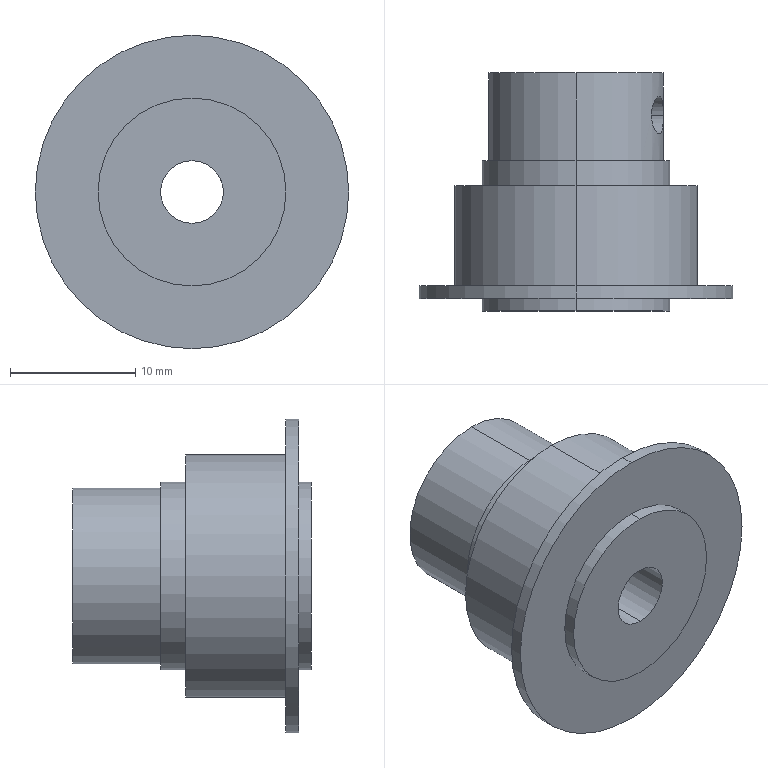Part | SolidWorks | features 3DProfileFeature 1, BaseBody 1, HoleWzd 1 | 1 solid | 20 faces | box 25 x 19 x 25 mm | volume 4058 mm3 | cylinder 14 | plane 6 | commonest cylinder face diameters 15 x4 3 x2 5 x2 14 x2 19.4 x2 25 x2
STEP:
#1=CARTESIAN_POINT('',(1.426,14.633,2.053));
#2=VERTEX_POINT('',#1);
#3=CARTESIAN_POINT('',(2.37,14.633,-0.7943));
#4=VERTEX_POINT('',#3);
#5=CARTESIAN_POINT('',(1.426,14.633,2.053));
#6=CARTESIAN_POINT('',(1.426,14.531,2.053));
#7=CARTESIAN_POINT('',(1.437,14.431,2.046));
#8=CARTESIAN_POINT('',(1.477,14.236,2.017));
#9=CARTESIAN_POINT('',(1.506,14.14,1.996));
#10=CARTESIAN_POINT('',(1.614,13.87,1.912));
#11=CARTESIAN_POINT('',(1.711,13.709,1.829));
#12=CARTESIAN_POINT('',(1.865,13.506,1.666));
#13=CARTESIAN_POINT('',(1.919,13.444,1.605));
#14=CARTESIAN_POINT('',(2.023,13.336,1.471));
#15=CARTESIAN_POINT('',(2.074,13.29,1.399));
#16=CARTESIAN_POINT('',(2.173,13.213,1.24));
#17=CARTESIAN_POINT('',(2.22,13.183,1.155));
#18=CARTESIAN_POINT('',(2.303,13.143,0.9773));
#19=CARTESIAN_POINT('',(2.341,13.133,0.8843));
#20=CARTESIAN_POINT('',(2.405,13.133,0.6911));
#21=CARTESIAN_POINT('',(2.43,13.143,0.5944));
#22=CARTESIAN_POINT('',(2.47,13.183,0.401));
#23=CARTESIAN_POINT('',(2.483,13.213,0.3036));
#24=CARTESIAN_POINT('',(2.507,13.328,0.0251));
#25=CARTESIAN_POINT('',(2.5,13.439,-0.1488));
#26=CARTESIAN_POINT('',(2.473,13.642,-0.3709));
#27=CARTESIAN_POINT('',(2.462,13.717,-0.4397));
#28=CARTESIAN_POINT('',(2.437,13.876,-0.5603));
#29=CARTESIAN_POINT('',(2.424,13.961,-0.6128));
#30=CARTESIAN_POINT('',(2.4,14.141,-0.7006));
#31=CARTESIAN_POINT('',(2.389,14.237,-0.7355));
#32=CARTESIAN_POINT('',(2.375,14.431,-0.782));
#33=CARTESIAN_POINT('',(2.37,14.531,-0.7943));
#34=CARTESIAN_POINT('',(2.37,14.633,-0.7943));
#35=B_SPLINE_CURVE_WITH_KNOTS('',3,(#5,#6,#7,#8,#9,#10,#11,#12,#13,#14,#15,#16,#17,#18,#19,#20,#21,#22,#23,#24,#25,#26,#27,#28,#29,#30,#31,#32,#33,#34),.UNSPECIFIED.,.F.,.F.,(4,2,2,2,2,2,2,2,2,2,2,2,2,2,4),(0.00481,0.00511,0.005411,0.006011,0.006311,0.006611,0.006911,0.007211,0.007511,0.007811,0.008412,0.008712,0.009012,0.009312,0.009612),.UNSPECIFIED.);
#36=EDGE_CURVE('',#2,#4,#35,.T.);
#37=ORIENTED_EDGE('',*,*,#36,.F.);
#38=CARTESIAN_POINT('',(6.018,14.633,3.576));
#39=VERTEX_POINT('',#38);
#40=CARTESIAN_POINT('',(6.172,14.633,3.627));
#41=DIRECTION('',(0.9492,0.,0.3147));
#42=VECTOR('',#41,1000.);
#43=LINE('',#40,#42);
#44=EDGE_CURVE('',#2,#39,#43,.T.);
#45=ORIENTED_EDGE('',*,*,#44,.T.);
#46=CARTESIAN_POINT('',(6.962,14.633,0.7282));
#47=VERTEX_POINT('',#46);
#48=CARTESIAN_POINT('',(6.962,14.633,0.7282));
#49=CARTESIAN_POINT('',(6.962,14.533,0.7282));
#50=CARTESIAN_POINT('',(6.961,14.436,0.7382));
#51=CARTESIAN_POINT('',(6.957,14.244,0.7771));
#52=CARTESIAN_POINT('',(6.953,14.148,0.8065));
#53=CARTESIAN_POINT('',(6.944,13.967,0.8829));
#54=CARTESIAN_POINT('',(6.938,13.881,0.9295));
#55=CARTESIAN_POINT('',(6.923,13.718,1.039));
#56=CARTESIAN_POINT('',(6.913,13.641,1.102));
#57=CARTESIAN_POINT('',(6.878,13.434,1.309));
#58=CARTESIAN_POINT('',(6.845,13.322,1.474));
#59=CARTESIAN_POINT('',(6.76,13.173,1.826));
#60=CARTESIAN_POINT('',(6.706,13.133,2.016));
#61=CARTESIAN_POINT('',(6.614,13.133,2.296));
#62=CARTESIAN_POINT('',(6.58,13.143,2.39));
#63=CARTESIAN_POINT('',(6.512,13.181,2.57));
#64=CARTESIAN_POINT('',(6.477,13.209,2.657));
#65=CARTESIAN_POINT('',(6.37,13.323,2.909));
#66=CARTESIAN_POINT('',(6.298,13.433,3.059));
#67=CARTESIAN_POINT('',(6.202,13.642,3.247));
#68=CARTESIAN_POINT('',(6.172,13.717,3.303));
#69=CARTESIAN_POINT('',(6.119,13.88,3.4));
#70=CARTESIAN_POINT('',(6.096,13.967,3.441));
#71=CARTESIAN_POINT('',(6.058,14.149,3.508));
#72=CARTESIAN_POINT('',(6.043,14.242,3.533));
#73=CARTESIAN_POINT('',(6.023,14.435,3.567));
#74=CARTESIAN_POINT('',(6.018,14.535,3.576));
#75=CARTESIAN_POINT('',(6.018,14.633,3.576));
#76=B_SPLINE_CURVE_WITH_KNOTS('',3,(#48,#49,#50,#51,#52,#53,#54,#55,#56,#57,#58,#59,#60,#61,#62,#63,#64,#65,#66,#67,#68,#69,#70,#71,#72,#73,#74,#75),.UNSPECIFIED.,.F.,.F.,(4,2,2,2,2,2,2,2,2,2,2,2,2,4),(0.,0.000294,0.0005879,0.0008819,0.001176,0.001764,0.002352,0.002646,0.00294,0.003527,0.003821,0.004115,0.004409,0.004703),.UNSPECIFIED.);
#77=EDGE_CURVE('',#47,#39,#76,.T.);
#78=ORIENTED_EDGE('',*,*,#77,.F.);
#79=CARTESIAN_POINT('',(7.116,14.633,0.7794));
#80=DIRECTION('',(0.9492,0.,0.3147));
#81=VECTOR('',#80,1000.);
#82=LINE('',#79,#81);
#83=EDGE_CURVE('',#4,#47,#82,.T.);
#84=ORIENTED_EDGE('',*,*,#83,.F.);
#85=EDGE_LOOP('',(#37,#45,#78,#84));
#86=FACE_OUTER_BOUND('',#85,.T.);
#87=CARTESIAN_POINT('',(6.644,14.633,2.203));
#88=DIRECTION('',(0.9492,0.,0.3147));
#89=DIRECTION('',(0.3147,0.,-0.9492));
#90=AXIS2_PLACEMENT_3D('',#87,#88,#89);
#91=CYLINDRICAL_SURFACE('',#90,1.5);
#92=ADVANCED_FACE('',(#86),#91,.F.);
#93=CARTESIAN_POINT('',(0.,-1.,-2.5));
#94=VERTEX_POINT('',#93);
#95=CARTESIAN_POINT('',(0.,-1.,2.5));
#96=VERTEX_POINT('',#95);
#97=CARTESIAN_POINT('',(0.,-1.,0.));
#98=DIRECTION('',(0.,1.,0.));
#99=DIRECTION('',(0.,0.,1.));
#100=AXIS2_PLACEMENT_3D('',#97,#98,#99);
#101=CIRCLE('',#100,2.5);
#102=EDGE_CURVE('',#94,#96,#101,.T.);
#103=ORIENTED_EDGE('',*,*,#102,.F.);
#104=CARTESIAN_POINT('',(0.,18.,-2.5));
#105=VERTEX_POINT('',#104);
#106=CARTESIAN_POINT('',(0.,-1.,-2.5));
#107=DIRECTION('',(0.,1.,0.));
#108=VECTOR('',#107,1000.);
#109=LINE('',#106,#108);
#110=EDGE_CURVE('',#94,#105,#109,.T.);
#111=ORIENTED_EDGE('',*,*,#110,.T.);
#112=CARTESIAN_POINT('',(0.,18.,2.5));
#113=VERTEX_POINT('',#112);
#114=CARTESIAN_POINT('',(0.,18.,0.));
#115=DIRECTION('',(0.,1.,0.));
#116=DIRECTION('',(0.,0.,1.));
#117=AXIS2_PLACEMENT_3D('',#114,#115,#116);
#118=CIRCLE('',#117,2.5);
#119=EDGE_CURVE('',#105,#113,#118,.T.);
#120=ORIENTED_EDGE('',*,*,#119,.T.);
#121=CARTESIAN_POINT('',(0.,-1.,2.5));
#122=DIRECTION('',(0.,1.,0.));
#123=VECTOR('',#122,1000.);
#124=LINE('',#121,#123);
#125=EDGE_CURVE('',#96,#113,#124,.T.);
#126=ORIENTED_EDGE('',*,*,#125,.F.);
#127=EDGE_LOOP('',(#103,#111,#120,#126));
#128=FACE_OUTER_BOUND('',#127,.T.);
#129=CARTESIAN_POINT('',(0.,-1.,0.));
#130=DIRECTION('',(0.,1.,0.));
#131=DIRECTION('',(0.,0.,1.));
#132=AXIS2_PLACEMENT_3D('',#129,#130,#131);
#133=CYLINDRICAL_SURFACE('',#132,2.5);
#134=ADVANCED_FACE('',(#128),#133,.F.);
#135=ORIENTED_EDGE('',*,*,#77,.T.);
#136=CARTESIAN_POINT('',(6.018,14.633,3.576));
#137=CARTESIAN_POINT('',(6.018,14.829,3.576));
#138=CARTESIAN_POINT('',(6.039,15.027,3.541));
#139=CARTESIAN_POINT('',(6.115,15.388,3.408));
#140=CARTESIAN_POINT('',(6.17,15.555,3.309));
#141=CARTESIAN_POINT('',(6.265,15.762,3.123));
#142=CARTESIAN_POINT('',(6.3,15.825,3.053));
#143=CARTESIAN_POINT('',(6.369,15.934,2.905));
#144=CARTESIAN_POINT('',(6.405,15.98,2.826));
#145=CARTESIAN_POINT('',(6.512,16.094,2.574));
#146=CARTESIAN_POINT('',(6.582,16.133,2.392));
#147=CARTESIAN_POINT('',(6.675,16.133,2.11));
#148=CARTESIAN_POINT('',(6.704,16.123,2.017));
#149=CARTESIAN_POINT('',(6.757,16.085,1.831));
#150=CARTESIAN_POINT('',(6.781,16.056,1.739));
#151=CARTESIAN_POINT('',(6.846,15.943,1.474));
#152=CARTESIAN_POINT('',(6.878,15.832,1.309));
#153=CARTESIAN_POINT('',(6.925,15.556,1.034));
#154=CARTESIAN_POINT('',(6.94,15.39,0.9212));
#155=CARTESIAN_POINT('',(6.958,15.029,0.7691));
#156=CARTESIAN_POINT('',(6.962,14.832,0.7282));
#157=CARTESIAN_POINT('',(6.962,14.633,0.7282));
#158=B_SPLINE_CURVE_WITH_KNOTS('',3,(#136,#137,#138,#139,#140,#141,#142,#143,#144,#145,#146,#147,#148,#149,#150,#151,#152,#153,#154,#155,#156,#157),.UNSPECIFIED.,.F.,.F.,(4,2,2,2,2,2,2,2,2,2,4),(0.004703,0.005291,0.005879,0.006173,0.006467,0.007054,0.007348,0.007642,0.00823,0.008818,0.009405),.UNSPECIFIED.);
#159=EDGE_CURVE('',#39,#47,#158,.T.);
#160=ORIENTED_EDGE('',*,*,#159,.T.);
#161=EDGE_LOOP('',(#135,#160));
#162=FACE_BOUND('',#161,.T.);
#163=CARTESIAN_POINT('',(0.,18.,7.));
#164=VERTEX_POINT('',#163);
#165=CARTESIAN_POINT('',(0.,18.,-7.));
#166=VERTEX_POINT('',#165);
#167=CARTESIAN_POINT('',(0.,18.,0.));
#168=DIRECTION('',(0.,1.,0.));
#169=DIRECTION('',(0.,0.,1.));
#170=AXIS2_PLACEMENT_3D('',#167,#168,#169);
#171=CIRCLE('',#170,7.);
#172=EDGE_CURVE('',#164,#166,#171,.T.);
#173=ORIENTED_EDGE('',*,*,#172,.F.);
#174=CARTESIAN_POINT('',(0.,11.,7.));
#175=VERTEX_POINT('',#174);
#176=CARTESIAN_POINT('',(0.,18.,7.));
#177=DIRECTION('',(0.,-1.,0.));
#178=VECTOR('',#177,1000.);
#179=LINE('',#176,#178);
#180=EDGE_CURVE('',#164,#175,#179,.T.);
#181=ORIENTED_EDGE('',*,*,#180,.T.);
#182=CARTESIAN_POINT('',(0.,11.,-7.));
#183=VERTEX_POINT('',#182);
#184=CARTESIAN_POINT('',(0.,11.,0.));
#185=DIRECTION('',(0.,1.,0.));
#186=DIRECTION('',(0.,0.,1.));
#187=AXIS2_PLACEMENT_3D('',#184,#185,#186);
#188=CIRCLE('',#187,7.);
#189=EDGE_CURVE('',#175,#183,#188,.T.);
#190=ORIENTED_EDGE('',*,*,#189,.T.);
#191=CARTESIAN_POINT('',(0.,18.,-7.));
#192=DIRECTION('',(0.,-1.,0.));
#193=VECTOR('',#192,1000.);
#194=LINE('',#191,#193);
#195=EDGE_CURVE('',#166,#183,#194,.T.);
#196=ORIENTED_EDGE('',*,*,#195,.F.);
#197=EDGE_LOOP('',(#173,#181,#190,#196));
#198=FACE_OUTER_BOUND('',#197,.T.);
#199=CARTESIAN_POINT('',(0.,18.,0.));
#200=DIRECTION('',(0.,-1.,0.));
#201=DIRECTION('',(0.,0.,-1.));
#202=AXIS2_PLACEMENT_3D('',#199,#200,#201);
#203=CYLINDRICAL_SURFACE('',#202,7.);
#204=ADVANCED_FACE('',(#162,#198),#203,.T.);
#205=CARTESIAN_POINT('',(0.,11.,7.5));
#206=VERTEX_POINT('',#205);
#207=CARTESIAN_POINT('',(0.,11.,-7.5));
#208=VERTEX_POINT('',#207);
#209=CARTESIAN_POINT('',(0.,11.,0.));
#210=DIRECTION('',(0.,1.,0.));
#211=DIRECTION('',(0.,0.,1.));
#212=AXIS2_PLACEMENT_3D('',#209,#210,#211);
#213=CIRCLE('',#212,7.5);
#214=EDGE_CURVE('',#206,#208,#213,.T.);
#215=ORIENTED_EDGE('',*,*,#214,.F.);
#216=CARTESIAN_POINT('',(0.,9.,7.5));
#217=VERTEX_POINT('',#216);
#218=CARTESIAN_POINT('',(0.,11.,7.5));
#219=DIRECTION('',(0.,-1.,0.));
#220=VECTOR('',#219,1000.);
#221=LINE('',#218,#220);
#222=EDGE_CURVE('',#206,#217,#221,.T.);
#223=ORIENTED_EDGE('',*,*,#222,.T.);
#224=CARTESIAN_POINT('',(0.,9.,-7.5));
#225=VERTEX_POINT('',#224);
#226=CARTESIAN_POINT('',(0.,9.,0.));
#227=DIRECTION('',(0.,1.,0.));
#228=DIRECTION('',(0.,0.,1.));
#229=AXIS2_PLACEMENT_3D('',#226,#227,#228);
#230=CIRCLE('',#229,7.5);
#231=EDGE_CURVE('',#217,#225,#230,.T.);
#232=ORIENTED_EDGE('',*,*,#231,.T.);
#233=CARTESIAN_POINT('',(0.,11.,-7.5));
#234=DIRECTION('',(0.,-1.,0.));
#235=VECTOR('',#234,1000.);
#236=LINE('',#233,#235);
#237=EDGE_CURVE('',#208,#225,#236,.T.);
#238=ORIENTED_EDGE('',*,*,#237,.F.);
#239=EDGE_LOOP('',(#215,#223,#232,#238));
#240=FACE_OUTER_BOUND('',#239,.T.);
#241=CARTESIAN_POINT('',(0.,11.,0.));
#242=DIRECTION('',(0.,-1.,0.));
#243=DIRECTION('',(0.,0.,-1.));
#244=AXIS2_PLACEMENT_3D('',#241,#242,#243);
#245=CYLINDRICAL_SURFACE('',#244,7.5);
#246=ADVANCED_FACE('',(#240),#245,.T.);
#247=CARTESIAN_POINT('',(0.,9.,9.7));
#248=VERTEX_POINT('',#247);
#249=CARTESIAN_POINT('',(0.,9.,-9.7));
#250=VERTEX_POINT('',#249);
#251=CARTESIAN_POINT('',(0.,9.,0.));
#252=DIRECTION('',(0.,1.,0.));
#253=DIRECTION('',(0.,0.,1.));
#254=AXIS2_PLACEMENT_3D('',#251,#252,#253);
#255=CIRCLE('',#254,9.7);
#256=EDGE_CURVE('',#248,#250,#255,.T.);
#257=ORIENTED_EDGE('',*,*,#256,.F.);
#258=CARTESIAN_POINT('',(0.,1.,9.7));
#259=VERTEX_POINT('',#258);
#260=CARTESIAN_POINT('',(0.,9.,9.7));
#261=DIRECTION('',(0.,-1.,0.));
#262=VECTOR('',#261,1000.);
#263=LINE('',#260,#262);
#264=EDGE_CURVE('',#248,#259,#263,.T.);
#265=ORIENTED_EDGE('',*,*,#264,.T.);
#266=CARTESIAN_POINT('',(0.,1.,-9.7));
#267=VERTEX_POINT('',#266);
#268=CARTESIAN_POINT('',(0.,1.,0.));
#269=DIRECTION('',(0.,1.,0.));
#270=DIRECTION('',(0.,0.,1.));
#271=AXIS2_PLACEMENT_3D('',#268,#269,#270);
#272=CIRCLE('',#271,9.7);
#273=EDGE_CURVE('',#259,#267,#272,.T.);
#274=ORIENTED_EDGE('',*,*,#273,.T.);
#275=CARTESIAN_POINT('',(0.,9.,-9.7));
#276=DIRECTION('',(0.,-1.,0.));
#277=VECTOR('',#276,1000.);
#278=LINE('',#275,#277);
#279=EDGE_CURVE('',#250,#267,#278,.T.);
#280=ORIENTED_EDGE('',*,*,#279,.F.);
#281=EDGE_LOOP('',(#257,#265,#274,#280));
#282=FACE_OUTER_BOUND('',#281,.T.);
#283=CARTESIAN_POINT('',(0.,9.,0.));
#284=DIRECTION('',(0.,-1.,0.));
#285=DIRECTION('',(0.,0.,-1.));
#286=AXIS2_PLACEMENT_3D('',#283,#284,#285);
#287=CYLINDRICAL_SURFACE('',#286,9.7);
#288=ADVANCED_FACE('',(#282),#287,.T.);
#289=CARTESIAN_POINT('',(0.,-1.,-7.5));
#290=VERTEX_POINT('',#289);
#291=CARTESIAN_POINT('',(0.,-1.,7.5));
#292=VERTEX_POINT('',#291);
#293=CARTESIAN_POINT('',(0.,-1.,0.));
#294=DIRECTION('',(0.,-1.,0.));
#295=DIRECTION('',(0.,0.,-1.));
#296=AXIS2_PLACEMENT_3D('',#293,#294,#295);
#297=CIRCLE('',#296,7.5);
#298=EDGE_CURVE('',#290,#292,#297,.T.);
#299=ORIENTED_EDGE('',*,*,#298,.F.);
#300=CARTESIAN_POINT('',(0.,0.,-7.5));
#301=VERTEX_POINT('',#300);
#302=CARTESIAN_POINT('',(0.,-1.,-7.5));
#303=DIRECTION('',(0.,1.,0.));
#304=VECTOR('',#303,1000.);
#305=LINE('',#302,#304);
#306=EDGE_CURVE('',#290,#301,#305,.T.);
#307=ORIENTED_EDGE('',*,*,#306,.T.);
#308=CARTESIAN_POINT('',(0.,0.,7.5));
#309=VERTEX_POINT('',#308);
#310=CARTESIAN_POINT('',(0.,0.,0.));
#311=DIRECTION('',(0.,-1.,0.));
#312=DIRECTION('',(0.,0.,1.));
#313=AXIS2_PLACEMENT_3D('',#310,#311,#312);
#314=CIRCLE('',#313,7.5);
#315=EDGE_CURVE('',#301,#309,#314,.T.);
#316=ORIENTED_EDGE('',*,*,#315,.T.);
#317=CARTESIAN_POINT('',(0.,-1.,7.5));
#318=DIRECTION('',(0.,1.,0.));
#319=VECTOR('',#318,1000.);
#320=LINE('',#317,#319);
#321=EDGE_CURVE('',#292,#309,#320,.T.);
#322=ORIENTED_EDGE('',*,*,#321,.F.);
#323=EDGE_LOOP('',(#299,#307,#316,#322));
#324=FACE_OUTER_BOUND('',#323,.T.);
#325=CARTESIAN_POINT('',(0.,-1.,0.));
#326=DIRECTION('',(0.,1.,0.));
#327=DIRECTION('',(0.,0.,1.));
#328=AXIS2_PLACEMENT_3D('',#325,#326,#327);
#329=CYLINDRICAL_SURFACE('',#328,7.5);
#330=ADVANCED_FACE('',(#324),#329,.T.);
#331=CARTESIAN_POINT('',(0.,1.,12.5));
#332=VERTEX_POINT('',#331);
#333=CARTESIAN_POINT('',(0.,1.,-12.5));
#334=VERTEX_POINT('',#333);
#335=CARTESIAN_POINT('',(0.,1.,0.));
#336=DIRECTION('',(0.,1.,0.));
#337=DIRECTION('',(0.,0.,1.));
#338=AXIS2_PLACEMENT_3D('',#335,#336,#337);
#339=CIRCLE('',#338,12.5);
#340=EDGE_CURVE('',#332,#334,#339,.T.);
#341=ORIENTED_EDGE('',*,*,#340,.F.);
#342=CARTESIAN_POINT('',(0.,0.,12.5));
#343=VERTEX_POINT('',#342);
#344=CARTESIAN_POINT('',(0.,1.,12.5));
#345=DIRECTION('',(0.,-1.,0.));
#346=VECTOR('',#345,1000.);
#347=LINE('',#344,#346);
#348=EDGE_CURVE('',#332,#343,#347,.T.);
#349=ORIENTED_EDGE('',*,*,#348,.T.);
#350=CARTESIAN_POINT('',(0.,0.,-12.5));
#351=VERTEX_POINT('',#350);
#352=CARTESIAN_POINT('',(0.,0.,0.));
#353=DIRECTION('',(0.,1.,0.));
#354=DIRECTION('',(0.,0.,1.));
#355=AXIS2_PLACEMENT_3D('',#352,#353,#354);
#356=CIRCLE('',#355,12.5);
#357=EDGE_CURVE('',#343,#351,#356,.T.);
#358=ORIENTED_EDGE('',*,*,#357,.T.);
#359=CARTESIAN_POINT('',(0.,1.,-12.5));
#360=DIRECTION('',(0.,-1.,0.));
#361=VECTOR('',#360,1000.);
#362=LINE('',#359,#361);
#363=EDGE_CURVE('',#334,#351,#362,.T.);
#364=ORIENTED_EDGE('',*,*,#363,.F.);
#365=EDGE_LOOP('',(#341,#349,#358,#364));
#366=FACE_OUTER_BOUND('',#365,.T.);
#367=CARTESIAN_POINT('',(0.,1.,0.));
#368=DIRECTION('',(0.,-1.,0.));
#369=DIRECTION('',(0.,0.,-1.));
#370=AXIS2_PLACEMENT_3D('',#367,#368,#369);
#371=CYLINDRICAL_SURFACE('',#370,12.5);
#372=ADVANCED_FACE('',(#366),#371,.T.);
#373=CARTESIAN_POINT('',(0.,11.,0.));
#374=DIRECTION('',(0.,1.,0.));
#375=DIRECTION('',(0.,0.,1.));
#376=AXIS2_PLACEMENT_3D('',#373,#374,#375);
#377=CIRCLE('',#376,7.5);
#378=EDGE_CURVE('',#208,#206,#377,.T.);
#379=ORIENTED_EDGE('',*,*,#378,.T.);
#380=ORIENTED_EDGE('',*,*,#214,.T.);
#381=EDGE_LOOP('',(#379,#380));
#382=FACE_OUTER_BOUND('',#381,.T.);
#383=CARTESIAN_POINT('',(0.,11.,0.));
#384=DIRECTION('',(0.,1.,0.));
#385=DIRECTION('',(0.,0.,1.));
#386=AXIS2_PLACEMENT_3D('',#383,#384,#385);
#387=CIRCLE('',#386,7.);
#388=EDGE_CURVE('',#183,#175,#387,.T.);
#389=ORIENTED_EDGE('',*,*,#388,.F.);
#390=ORIENTED_EDGE('',*,*,#189,.F.);
#391=EDGE_LOOP('',(#389,#390));
#392=FACE_BOUND('',#391,.T.);
#393=CARTESIAN_POINT('',(0.,11.,0.));
#394=DIRECTION('',(0.,1.,0.));
#395=DIRECTION('',(0.,0.,1.));
#396=AXIS2_PLACEMENT_3D('',#393,#394,#395);
#397=PLANE('',#396);
#398=ADVANCED_FACE('',(#382,#392),#397,.T.);
#399=CARTESIAN_POINT('',(0.,9.,0.));
#400=DIRECTION('',(0.,1.,0.));
#401=DIRECTION('',(0.,0.,1.));
#402=AXIS2_PLACEMENT_3D('',#399,#400,#401);
#403=CIRCLE('',#402,9.7);
#404=EDGE_CURVE('',#250,#248,#403,.T.);
#405=ORIENTED_EDGE('',*,*,#404,.T.);
#406=ORIENTED_EDGE('',*,*,#256,.T.);
#407=EDGE_LOOP('',(#405,#406));
#408=FACE_OUTER_BOUND('',#407,.T.);
#409=CARTESIAN_POINT('',(0.,9.,0.));
#410=DIRECTION('',(0.,1.,0.));
#411=DIRECTION('',(0.,0.,1.));
#412=AXIS2_PLACEMENT_3D('',#409,#410,#411);
#413=CIRCLE('',#412,7.5);
#414=EDGE_CURVE('',#225,#217,#413,.T.);
#415=ORIENTED_EDGE('',*,*,#414,.F.);
#416=ORIENTED_EDGE('',*,*,#231,.F.);
#417=EDGE_LOOP('',(#415,#416));
#418=FACE_BOUND('',#417,.T.);
#419=CARTESIAN_POINT('',(0.,9.,0.));
#420=DIRECTION('',(0.,1.,0.));
#421=DIRECTION('',(0.,0.,1.));
#422=AXIS2_PLACEMENT_3D('',#419,#420,#421);
#423=PLANE('',#422);
#424=ADVANCED_FACE('',(#408,#418),#423,.T.);
#425=CARTESIAN_POINT('',(0.,1.,0.));
#426=DIRECTION('',(0.,1.,0.));
#427=DIRECTION('',(0.,0.,1.));
#428=AXIS2_PLACEMENT_3D('',#425,#426,#427);
#429=CIRCLE('',#428,12.5);
#430=EDGE_CURVE('',#334,#332,#429,.T.);
#431=ORIENTED_EDGE('',*,*,#430,.T.);
#432=ORIENTED_EDGE('',*,*,#340,.T.);
#433=EDGE_LOOP('',(#431,#432));
#434=FACE_OUTER_BOUND('',#433,.T.);
#435=CARTESIAN_POINT('',(0.,1.,0.));
#436=DIRECTION('',(0.,1.,0.));
#437=DIRECTION('',(0.,0.,1.));
#438=AXIS2_PLACEMENT_3D('',#435,#436,#437);
#439=CIRCLE('',#438,9.7);
#440=EDGE_CURVE('',#267,#259,#439,.T.);
#441=ORIENTED_EDGE('',*,*,#440,.F.);
#442=ORIENTED_EDGE('',*,*,#273,.F.);
#443=EDGE_LOOP('',(#441,#442));
#444=FACE_BOUND('',#443,.T.);
#445=CARTESIAN_POINT('',(0.,1.,0.));
#446=DIRECTION('',(0.,1.,0.));
#447=DIRECTION('',(0.,0.,1.));
#448=AXIS2_PLACEMENT_3D('',#445,#446,#447);
#449=PLANE('',#448);
#450=ADVANCED_FACE('',(#434,#444),#449,.T.);
#451=CARTESIAN_POINT('',(0.,0.,0.));
#452=DIRECTION('',(0.,1.,0.));
#453=DIRECTION('',(0.,0.,1.));
#454=AXIS2_PLACEMENT_3D('',#451,#452,#453);
#455=CIRCLE('',#454,12.5);
#456=EDGE_CURVE('',#351,#343,#455,.T.);
#457=ORIENTED_EDGE('',*,*,#456,.F.);
#458=ORIENTED_EDGE('',*,*,#357,.F.);
#459=EDGE_LOOP('',(#457,#458));
#460=FACE_OUTER_BOUND('',#459,.T.);
#461=CARTESIAN_POINT('',(0.,0.,0.));
#462=DIRECTION('',(0.,-1.,0.));
#463=DIRECTION('',(0.,0.,1.));
#464=AXIS2_PLACEMENT_3D('',#461,#462,#463);
#465=CIRCLE('',#464,7.5);
#466=EDGE_CURVE('',#309,#301,#465,.T.);
#467=ORIENTED_EDGE('',*,*,#466,.F.);
#468=ORIENTED_EDGE('',*,*,#315,.F.);
#469=EDGE_LOOP('',(#467,#468));
#470=FACE_BOUND('',#469,.T.);
#471=CARTESIAN_POINT('',(0.,0.,0.));
#472=DIRECTION('',(0.,1.,0.));
#473=DIRECTION('',(0.,0.,1.));
#474=AXIS2_PLACEMENT_3D('',#471,#472,#473);
#475=PLANE('',#474);
#476=ADVANCED_FACE('',(#460,#470),#475,.F.);
#477=ORIENTED_EDGE('',*,*,#348,.F.);
#478=ORIENTED_EDGE('',*,*,#430,.F.);
#479=ORIENTED_EDGE('',*,*,#363,.T.);
#480=ORIENTED_EDGE('',*,*,#456,.T.);
#481=EDGE_LOOP('',(#477,#478,#479,#480));
#482=FACE_OUTER_BOUND('',#481,.T.);
#483=CARTESIAN_POINT('',(0.,1.,0.));
#484=DIRECTION('',(0.,-1.,0.));
#485=DIRECTION('',(0.,0.,-1.));
#486=AXIS2_PLACEMENT_3D('',#483,#484,#485);
#487=CYLINDRICAL_SURFACE('',#486,12.5);
#488=ADVANCED_FACE('',(#482),#487,.T.);
#489=ORIENTED_EDGE('',*,*,#306,.F.);
#490=CARTESIAN_POINT('',(0.,-1.,0.));
#491=DIRECTION('',(0.,-1.,0.));
#492=DIRECTION('',(0.,0.,-1.));
#493=AXIS2_PLACEMENT_3D('',#490,#491,#492);
#494=CIRCLE('',#493,7.5);
#495=EDGE_CURVE('',#292,#290,#494,.T.);
#496=ORIENTED_EDGE('',*,*,#495,.F.);
#497=ORIENTED_EDGE('',*,*,#321,.T.);
#498=ORIENTED_EDGE('',*,*,#466,.T.);
#499=EDGE_LOOP('',(#489,#496,#497,#498));
#500=FACE_OUTER_BOUND('',#499,.T.);
#501=CARTESIAN_POINT('',(0.,-1.,0.));
#502=DIRECTION('',(0.,1.,0.));
#503=DIRECTION('',(0.,0.,1.));
#504=AXIS2_PLACEMENT_3D('',#501,#502,#503);
#505=CYLINDRICAL_SURFACE('',#504,7.5);
#506=ADVANCED_FACE('',(#500),#505,.T.);
#507=CARTESIAN_POINT('',(0.,-1.,0.));
#508=DIRECTION('',(0.,1.,0.));
#509=DIRECTION('',(0.,0.,1.));
#510=AXIS2_PLACEMENT_3D('',#507,#508,#509);
#511=CIRCLE('',#510,2.5);
#512=EDGE_CURVE('',#96,#94,#511,.T.);
#513=ORIENTED_EDGE('',*,*,#512,.T.);
#514=ORIENTED_EDGE('',*,*,#102,.T.);
#515=EDGE_LOOP('',(#513,#514));
#516=FACE_BOUND('',#515,.T.);
#517=ORIENTED_EDGE('',*,*,#495,.T.);
#518=ORIENTED_EDGE('',*,*,#298,.T.);
#519=EDGE_LOOP('',(#517,#518));
#520=FACE_OUTER_BOUND('',#519,.T.);
#521=CARTESIAN_POINT('',(0.,-1.,0.));
#522=DIRECTION('',(0.,-1.,0.));
#523=DIRECTION('',(0.,0.,-1.));
#524=AXIS2_PLACEMENT_3D('',#521,#522,#523);
#525=PLANE('',#524);
#526=ADVANCED_FACE('',(#516,#520),#525,.T.);
#527=ORIENTED_EDGE('',*,*,#264,.F.);
#528=ORIENTED_EDGE('',*,*,#404,.F.);
#529=ORIENTED_EDGE('',*,*,#279,.T.);
#530=ORIENTED_EDGE('',*,*,#440,.T.);
#531=EDGE_LOOP('',(#527,#528,#529,#530));
#532=FACE_OUTER_BOUND('',#531,.T.);
#533=CARTESIAN_POINT('',(0.,9.,0.));
#534=DIRECTION('',(0.,-1.,0.));
#535=DIRECTION('',(0.,0.,-1.));
#536=AXIS2_PLACEMENT_3D('',#533,#534,#535);
#537=CYLINDRICAL_SURFACE('',#536,9.7);
#538=ADVANCED_FACE('',(#532),#537,.T.);
#539=ORIENTED_EDGE('',*,*,#222,.F.);
#540=ORIENTED_EDGE('',*,*,#378,.F.);
#541=ORIENTED_EDGE('',*,*,#237,.T.);
#542=ORIENTED_EDGE('',*,*,#414,.T.);
#543=EDGE_LOOP('',(#539,#540,#541,#542));
#544=FACE_OUTER_BOUND('',#543,.T.);
#545=CARTESIAN_POINT('',(0.,11.,0.));
#546=DIRECTION('',(0.,-1.,0.));
#547=DIRECTION('',(0.,0.,-1.));
#548=AXIS2_PLACEMENT_3D('',#545,#546,#547);
#549=CYLINDRICAL_SURFACE('',#548,7.5);
#550=ADVANCED_FACE('',(#544),#549,.T.);
#551=ORIENTED_EDGE('',*,*,#180,.F.);
#552=CARTESIAN_POINT('',(0.,18.,0.));
#553=DIRECTION('',(0.,1.,0.));
#554=DIRECTION('',(0.,0.,1.));
#555=AXIS2_PLACEMENT_3D('',#552,#553,#554);
#556=CIRCLE('',#555,7.);
#557=EDGE_CURVE('',#166,#164,#556,.T.);
#558=ORIENTED_EDGE('',*,*,#557,.F.);
#559=ORIENTED_EDGE('',*,*,#195,.T.);
#560=ORIENTED_EDGE('',*,*,#388,.T.);
#561=EDGE_LOOP('',(#551,#558,#559,#560));
#562=FACE_OUTER_BOUND('',#561,.T.);
#563=CARTESIAN_POINT('',(0.,18.,0.));
#564=DIRECTION('',(0.,-1.,0.));
#565=DIRECTION('',(0.,0.,-1.));
#566=AXIS2_PLACEMENT_3D('',#563,#564,#565);
#567=CYLINDRICAL_SURFACE('',#566,7.);
#568=ADVANCED_FACE('',(#562),#567,.T.);
#569=CARTESIAN_POINT('',(0.,18.,0.));
#570=DIRECTION('',(0.,1.,0.));
#571=DIRECTION('',(0.,0.,1.));
#572=AXIS2_PLACEMENT_3D('',#569,#570,#571);
#573=CIRCLE('',#572,2.5);
#574=EDGE_CURVE('',#113,#105,#573,.T.);
#575=ORIENTED_EDGE('',*,*,#574,.F.);
#576=ORIENTED_EDGE('',*,*,#119,.F.);
#577=EDGE_LOOP('',(#575,#576));
#578=FACE_BOUND('',#577,.T.);
#579=ORIENTED_EDGE('',*,*,#557,.T.);
#580=ORIENTED_EDGE('',*,*,#172,.T.);
#581=EDGE_LOOP('',(#579,#580));
#582=FACE_OUTER_BOUND('',#581,.T.);
#583=CARTESIAN_POINT('',(0.,18.,0.));
#584=DIRECTION('',(0.,1.,0.));
#585=DIRECTION('',(0.,0.,1.));
#586=AXIS2_PLACEMENT_3D('',#583,#584,#585);
#587=PLANE('',#586);
#588=ADVANCED_FACE('',(#578,#582),#587,.T.);
#589=ORIENTED_EDGE('',*,*,#110,.F.);
#590=ORIENTED_EDGE('',*,*,#512,.F.);
#591=ORIENTED_EDGE('',*,*,#125,.T.);
#592=ORIENTED_EDGE('',*,*,#574,.T.);
#593=EDGE_LOOP('',(#589,#590,#591,#592));
#594=FACE_OUTER_BOUND('',#593,.T.);
#595=CARTESIAN_POINT('',(2.37,14.633,-0.7943));
#596=CARTESIAN_POINT('',(2.37,14.735,-0.7943));
#597=CARTESIAN_POINT('',(2.375,14.834,-0.7821));
#598=CARTESIAN_POINT('',(2.39,15.029,-0.7354));
#599=CARTESIAN_POINT('',(2.4,15.125,-0.7004));
#600=CARTESIAN_POINT('',(2.436,15.395,-0.569));
#601=CARTESIAN_POINT('',(2.465,15.556,-0.4442));
#602=CARTESIAN_POINT('',(2.491,15.759,-0.2226));
#603=CARTESIAN_POINT('',(2.497,15.821,-0.1415));
#604=CARTESIAN_POINT('',(2.501,15.929,0.02824));
#605=CARTESIAN_POINT('',(2.499,15.976,0.1169));
#606=CARTESIAN_POINT('',(2.483,16.052,0.3017));
#607=CARTESIAN_POINT('',(2.47,16.082,0.3991));
#608=CARTESIAN_POINT('',(2.431,16.122,0.5919));
#609=CARTESIAN_POINT('',(2.406,16.133,0.6882));
#610=CARTESIAN_POINT('',(2.31,16.133,0.9764));
#611=CARTESIAN_POINT('',(2.223,16.092,1.16));
#612=CARTESIAN_POINT('',(2.026,15.938,1.477));
#613=CARTESIAN_POINT('',(1.916,15.827,1.612));
#614=CARTESIAN_POINT('',(1.711,15.557,1.829));
#615=CARTESIAN_POINT('',(1.614,15.395,1.912));
#616=CARTESIAN_POINT('',(1.507,15.126,1.995));
#617=CARTESIAN_POINT('',(1.477,15.03,2.017));
#618=CARTESIAN_POINT('',(1.437,14.835,2.046));
#619=CARTESIAN_POINT('',(1.426,14.735,2.053));
#620=CARTESIAN_POINT('',(1.426,14.633,2.053));
#621=B_SPLINE_CURVE_WITH_KNOTS('',3,(#595,#596,#597,#598,#599,#600,#601,#602,#603,#604,#605,#606,#607,#608,#609,#610,#611,#612,#613,#614,#615,#616,#617,#618,#619,#620),.UNSPECIFIED.,.F.,.F.,(4,2,2,2,2,2,2,2,2,2,2,2,4),(0.,0.0003006,0.0006013,0.001203,0.001503,0.001804,0.002105,0.002405,0.003006,0.003608,0.004209,0.00451,0.00481),.UNSPECIFIED.);
#622=EDGE_CURVE('',#4,#2,#621,.T.);
#623=ORIENTED_EDGE('',*,*,#622,.T.);
#624=ORIENTED_EDGE('',*,*,#36,.T.);
#625=EDGE_LOOP('',(#623,#624));
#626=FACE_BOUND('',#625,.T.);
#627=CARTESIAN_POINT('',(0.,-1.,0.));
#628=DIRECTION('',(0.,1.,0.));
#629=DIRECTION('',(0.,0.,1.));
#630=AXIS2_PLACEMENT_3D('',#627,#628,#629);
#631=CYLINDRICAL_SURFACE('',#630,2.5);
#632=ADVANCED_FACE('',(#594,#626),#631,.F.);
#633=ORIENTED_EDGE('',*,*,#44,.F.);
#634=ORIENTED_EDGE('',*,*,#622,.F.);
#635=ORIENTED_EDGE('',*,*,#83,.T.);
#636=ORIENTED_EDGE('',*,*,#159,.F.);
#637=EDGE_LOOP('',(#633,#634,#635,#636));
#638=FACE_OUTER_BOUND('',#637,.T.);
#639=CARTESIAN_POINT('',(6.644,14.633,2.203));
#640=DIRECTION('',(0.9492,0.,0.3147));
#641=DIRECTION('',(0.3147,0.,-0.9492));
#642=AXIS2_PLACEMENT_3D('',#639,#640,#641);
#643=CYLINDRICAL_SURFACE('',#642,1.5);
#644=ADVANCED_FACE('',(#638),#643,.F.);
#645=CLOSED_SHELL('',(#92,#134,#204,#246,#288,#330,#372,#398,#424,#450,#476,#488,#506,#526,#538,#550,#568,#588,#632,#644));
#646=MANIFOLD_SOLID_BREP('',#645);
#647=CARTESIAN_POINT('',(0.,0.,0.));
#648=DIRECTION('',(0.,0.,1.));
#649=DIRECTION('',(1.,0.,0.));
#650=AXIS2_PLACEMENT_3D('',#647,#648,#649);
#651=(LENGTH_UNIT()NAMED_UNIT(*)SI_UNIT(.MILLI.,.METRE.));
#652=UNCERTAINTY_MEASURE_WITH_UNIT(LENGTH_MEASURE(0.00001),#651,'','');
#653=(NAMED_UNIT(*)PLANE_ANGLE_UNIT()SI_UNIT($,.RADIAN.));
#654=(NAMED_UNIT(*)SI_UNIT($,.STERADIAN.)SOLID_ANGLE_UNIT());
#655=(GEOMETRIC_REPRESENTATION_CONTEXT(3)GLOBAL_UNCERTAINTY_ASSIGNED_CONTEXT((#652))GLOBAL_UNIT_ASSIGNED_CONTEXT((#651,#653,#654))REPRESENTATION_CONTEXT('',''));
#656=ADVANCED_BREP_SHAPE_REPRESENTATION('',(#646,#650),#655);